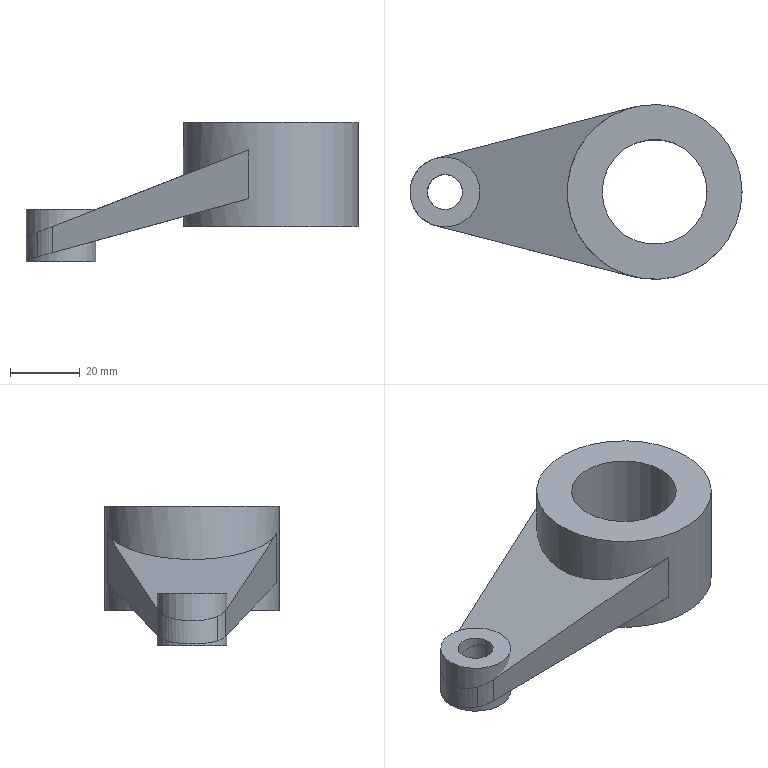Part | NX | features DATUM_CSYS 7, EXTRUDE 6, SKETCH 6, REPLACE_FACE 5, DATUM_PLANE 2 | 2 solids | 15 faces | box 95 x 50 x 40 mm | volume 53901 mm3 | plane 8 | cylinder 7 | commonest cylinder face diameters 20 x3 10 x2 30 x1 50 x1
STEP:
#1=CARTESIAN_POINT('',(5.,0.,13.029));
#2=VERTEX_POINT('',#1);
#3=CARTESIAN_POINT('',(0.,0.,11.079));
#4=DIRECTION('',(0.3634,0.,-0.9316));
#5=DIRECTION('',(0.9316,0.,0.3634));
#6=AXIS2_PLACEMENT_3D('',#3,#4,#5);
#7=ELLIPSE('',#6,5.367,5.);
#8=EDGE_CURVE('',#2,#2,#7,.F.);
#9=ORIENTED_EDGE('',*,*,#8,.F.);
#10=EDGE_LOOP('',(#9));
#11=FACE_BOUND('',#10,.T.);
#12=CARTESIAN_POINT('',(53.75,-24.206,32.048));
#13=VERTEX_POINT('',#12);
#14=CARTESIAN_POINT('',(53.75,24.206,32.048));
#15=VERTEX_POINT('',#14);
#16=CARTESIAN_POINT('',(60.,0.,34.486));
#17=DIRECTION('',(0.3634,0.,-0.9316));
#18=DIRECTION('',(-0.9316,0.,-0.3634));
#19=AXIS2_PLACEMENT_3D('',#16,#17,#18);
#20=ELLIPSE('',#19,26.835,25.);
#21=EDGE_CURVE('',#13,#15,#20,.T.);
#22=ORIENTED_EDGE('',*,*,#21,.T.);
#23=CARTESIAN_POINT('',(-2.5,9.682,10.103));
#24=VERTEX_POINT('',#23);
#25=CARTESIAN_POINT('',(-24.938,3.889,1.35));
#26=DIRECTION('',(0.9058,0.2339,0.3534));
#27=VECTOR('',#26,1000.);
#28=LINE('',#25,#27);
#29=EDGE_CURVE('',#24,#15,#28,.T.);
#30=ORIENTED_EDGE('',*,*,#29,.F.);
#31=CARTESIAN_POINT('',(-6.747,-7.381,8.447));
#32=VERTEX_POINT('',#31);
#33=CARTESIAN_POINT('',(0.,0.,11.079));
#34=DIRECTION('',(0.3634,0.,-0.9316));
#35=DIRECTION('',(-0.9316,0.,-0.3634));
#36=AXIS2_PLACEMENT_3D('',#33,#34,#35);
#37=ELLIPSE('',#36,10.734,10.);
#38=EDGE_CURVE('',#24,#32,#37,.F.);
#39=ORIENTED_EDGE('',*,*,#38,.T.);
#40=CARTESIAN_POINT('',(-2.5,-9.682,10.103));
#41=VERTEX_POINT('',#40);
#42=CARTESIAN_POINT('',(0.,0.,11.079));
#43=DIRECTION('',(0.3634,0.,-0.9316));
#44=DIRECTION('',(-0.9316,0.,-0.3634));
#45=AXIS2_PLACEMENT_3D('',#42,#43,#44);
#46=ELLIPSE('',#45,10.734,10.);
#47=EDGE_CURVE('',#32,#41,#46,.F.);
#48=ORIENTED_EDGE('',*,*,#47,.T.);
#49=CARTESIAN_POINT('',(-14.921,-6.475,5.258));
#50=DIRECTION('',(0.9058,-0.2339,0.3534));
#51=VECTOR('',#50,1000.);
#52=LINE('',#49,#51);
#53=EDGE_CURVE('',#41,#13,#52,.T.);
#54=ORIENTED_EDGE('',*,*,#53,.T.);
#55=EDGE_LOOP('',(#22,#30,#39,#48,#54));
#56=FACE_BOUND('',#55,.T.);
#57=CARTESIAN_POINT('',(-6.747,30.,8.447));
#58=DIRECTION('',(0.3634,0.,-0.9316));
#59=DIRECTION('',(-0.9316,0.,-0.3634));
#60=AXIS2_PLACEMENT_3D('',#57,#58,#59);
#61=PLANE('',#60);
#62=ADVANCED_FACE('',(#11,#56),#61,.F.);
#63=CARTESIAN_POINT('',(5.,0.,4.697));
#64=VERTEX_POINT('',#63);
#65=CARTESIAN_POINT('',(0.,0.,3.321));
#66=DIRECTION('',(-0.2654,0.,0.9641));
#67=DIRECTION('',(0.9641,0.,0.2654));
#68=AXIS2_PLACEMENT_3D('',#65,#66,#67);
#69=ELLIPSE('',#68,5.186,5.);
#70=EDGE_CURVE('',#64,#64,#69,.F.);
#71=ORIENTED_EDGE('',*,*,#70,.F.);
#72=EDGE_LOOP('',(#71));
#73=FACE_BOUND('',#72,.T.);
#74=CARTESIAN_POINT('',(53.75,24.206,18.117));
#75=VERTEX_POINT('',#74);
#76=CARTESIAN_POINT('',(-2.5,9.682,2.633));
#77=VERTEX_POINT('',#76);
#78=CARTESIAN_POINT('',(-17.591,5.786,-1.522));
#79=DIRECTION('',(-0.9356,-0.2416,-0.2575));
#80=VECTOR('',#79,1000.);
#81=LINE('',#78,#80);
#82=EDGE_CURVE('',#75,#77,#81,.T.);
#83=ORIENTED_EDGE('',*,*,#82,.F.);
#84=CARTESIAN_POINT('',(53.75,-24.206,18.117));
#85=VERTEX_POINT('',#84);
#86=CARTESIAN_POINT('',(60.,0.,19.837));
#87=DIRECTION('',(-0.2654,0.,0.9641));
#88=DIRECTION('',(-0.9641,0.,-0.2654));
#89=AXIS2_PLACEMENT_3D('',#86,#87,#88);
#90=ELLIPSE('',#89,25.93,25.);
#91=EDGE_CURVE('',#75,#85,#90,.T.);
#92=ORIENTED_EDGE('',*,*,#91,.T.);
#93=CARTESIAN_POINT('',(-2.5,-9.682,2.633));
#94=VERTEX_POINT('',#93);
#95=CARTESIAN_POINT('',(57.593,-25.198,19.175));
#96=DIRECTION('',(-0.9356,0.2416,-0.2575));
#97=VECTOR('',#96,1000.);
#98=LINE('',#95,#97);
#99=EDGE_CURVE('',#85,#94,#98,.T.);
#100=ORIENTED_EDGE('',*,*,#99,.T.);
#101=CARTESIAN_POINT('',(-6.747,-7.381,1.464));
#102=VERTEX_POINT('',#101);
#103=CARTESIAN_POINT('',(0.,0.,3.321));
#104=DIRECTION('',(-0.2654,0.,0.9641));
#105=DIRECTION('',(-0.9641,0.,-0.2654));
#106=AXIS2_PLACEMENT_3D('',#103,#104,#105);
#107=ELLIPSE('',#106,10.372,10.);
#108=EDGE_CURVE('',#94,#102,#107,.F.);
#109=ORIENTED_EDGE('',*,*,#108,.T.);
#110=CARTESIAN_POINT('',(0.,0.,3.321));
#111=DIRECTION('',(-0.2654,0.,0.9641));
#112=DIRECTION('',(-0.9641,0.,-0.2654));
#113=AXIS2_PLACEMENT_3D('',#110,#111,#112);
#114=ELLIPSE('',#113,10.372,10.);
#115=EDGE_CURVE('',#77,#102,#114,.T.);
#116=ORIENTED_EDGE('',*,*,#115,.F.);
#117=EDGE_LOOP('',(#83,#92,#100,#109,#116));
#118=FACE_BOUND('',#117,.T.);
#119=CARTESIAN_POINT('',(70.841,30.,22.822));
#120=DIRECTION('',(-0.2654,0.,0.9641));
#121=DIRECTION('',(0.9641,0.,0.2654));
#122=AXIS2_PLACEMENT_3D('',#119,#120,#121);
#123=PLANE('',#122);
#124=ADVANCED_FACE('',(#73,#118),#123,.F.);
#125=CARTESIAN_POINT('',(53.75,24.206,30.769));
#126=DIRECTION('',(0.,0.,-1.));
#127=VECTOR('',#126,1000.);
#128=LINE('',#125,#127);
#129=EDGE_CURVE('',#15,#75,#128,.T.);
#130=ORIENTED_EDGE('',*,*,#129,.F.);
#131=ORIENTED_EDGE('',*,*,#21,.F.);
#132=CARTESIAN_POINT('',(53.75,-24.206,30.769));
#133=DIRECTION('',(0.,0.,-1.));
#134=VECTOR('',#133,1000.);
#135=LINE('',#132,#134);
#136=EDGE_CURVE('',#13,#85,#135,.T.);
#137=ORIENTED_EDGE('',*,*,#136,.T.);
#138=ORIENTED_EDGE('',*,*,#91,.F.);
#139=EDGE_LOOP('',(#130,#131,#137,#138));
#140=FACE_BOUND('',#139,.T.);
#141=CARTESIAN_POINT('',(85.,0.,10.));
#142=VERTEX_POINT('',#141);
#143=CARTESIAN_POINT('',(60.,0.,10.));
#144=DIRECTION('',(0.,0.,1.));
#145=DIRECTION('',(1.,0.,0.));
#146=AXIS2_PLACEMENT_3D('',#143,#144,#145);
#147=CIRCLE('',#146,25.);
#148=EDGE_CURVE('',#142,#142,#147,.T.);
#149=ORIENTED_EDGE('',*,*,#148,.T.);
#150=EDGE_LOOP('',(#149));
#151=FACE_BOUND('',#150,.T.);
#152=CARTESIAN_POINT('',(85.,0.,40.));
#153=VERTEX_POINT('',#152);
#154=CARTESIAN_POINT('',(60.,0.,40.));
#155=DIRECTION('',(0.,0.,1.));
#156=DIRECTION('',(1.,0.,0.));
#157=AXIS2_PLACEMENT_3D('',#154,#155,#156);
#158=CIRCLE('',#157,25.);
#159=EDGE_CURVE('',#153,#153,#158,.T.);
#160=ORIENTED_EDGE('',*,*,#159,.F.);
#161=EDGE_LOOP('',(#160));
#162=FACE_BOUND('',#161,.T.);
#163=CARTESIAN_POINT('',(60.,0.,40.));
#164=DIRECTION('',(0.,0.,-1.));
#165=DIRECTION('',(-1.,0.,0.));
#166=AXIS2_PLACEMENT_3D('',#163,#164,#165);
#167=CYLINDRICAL_SURFACE('',#166,25.);
#168=ADVANCED_FACE('',(#140,#151,#162),#167,.T.);
#169=CARTESIAN_POINT('',(75.,0.,40.));
#170=VERTEX_POINT('',#169);
#171=CARTESIAN_POINT('',(60.,0.,40.));
#172=DIRECTION('',(0.,0.,1.));
#173=DIRECTION('',(1.,0.,0.));
#174=AXIS2_PLACEMENT_3D('',#171,#172,#173);
#175=CIRCLE('',#174,15.);
#176=EDGE_CURVE('',#170,#170,#175,.T.);
#177=ORIENTED_EDGE('',*,*,#176,.T.);
#178=EDGE_LOOP('',(#177));
#179=FACE_BOUND('',#178,.T.);
#180=CARTESIAN_POINT('',(75.,0.,10.));
#181=VERTEX_POINT('',#180);
#182=CARTESIAN_POINT('',(60.,0.,10.));
#183=DIRECTION('',(0.,0.,1.));
#184=DIRECTION('',(1.,0.,0.));
#185=AXIS2_PLACEMENT_3D('',#182,#183,#184);
#186=CIRCLE('',#185,15.);
#187=EDGE_CURVE('',#181,#181,#186,.T.);
#188=ORIENTED_EDGE('',*,*,#187,.F.);
#189=EDGE_LOOP('',(#188));
#190=FACE_BOUND('',#189,.T.);
#191=CARTESIAN_POINT('',(60.,0.,40.));
#192=DIRECTION('',(0.,0.,-1.));
#193=DIRECTION('',(-1.,0.,0.));
#194=AXIS2_PLACEMENT_3D('',#191,#192,#193);
#195=CYLINDRICAL_SURFACE('',#194,15.);
#196=ADVANCED_FACE('',(#179,#190),#195,.F.);
#197=ORIENTED_EDGE('',*,*,#159,.T.);
#198=EDGE_LOOP('',(#197));
#199=FACE_BOUND('',#198,.T.);
#200=ORIENTED_EDGE('',*,*,#176,.F.);
#201=EDGE_LOOP('',(#200));
#202=FACE_BOUND('',#201,.T.);
#203=CARTESIAN_POINT('',(60.,0.,40.));
#204=DIRECTION('',(0.,0.,1.));
#205=DIRECTION('',(1.,0.,0.));
#206=AXIS2_PLACEMENT_3D('',#203,#204,#205);
#207=PLANE('',#206);
#208=ADVANCED_FACE('',(#199,#202),#207,.T.);
#209=ORIENTED_EDGE('',*,*,#148,.F.);
#210=EDGE_LOOP('',(#209));
#211=FACE_BOUND('',#210,.T.);
#212=ORIENTED_EDGE('',*,*,#187,.T.);
#213=EDGE_LOOP('',(#212));
#214=FACE_BOUND('',#213,.T.);
#215=CARTESIAN_POINT('',(60.,0.,10.));
#216=DIRECTION('',(0.,0.,1.));
#217=DIRECTION('',(1.,0.,0.));
#218=AXIS2_PLACEMENT_3D('',#215,#216,#217);
#219=PLANE('',#218);
#220=ADVANCED_FACE('',(#211,#214),#219,.F.);
#221=CARTESIAN_POINT('',(-6.747,-7.381,4.955));
#222=DIRECTION('',(0.,0.,-1.));
#223=VECTOR('',#222,1000.);
#224=LINE('',#221,#223);
#225=EDGE_CURVE('',#102,#32,#224,.F.);
#226=ORIENTED_EDGE('',*,*,#225,.T.);
#227=ORIENTED_EDGE('',*,*,#38,.F.);
#228=CARTESIAN_POINT('',(-2.5,9.682,4.955));
#229=DIRECTION('',(0.,0.,-1.));
#230=VECTOR('',#229,1000.);
#231=LINE('',#228,#230);
#232=EDGE_CURVE('',#77,#24,#231,.F.);
#233=ORIENTED_EDGE('',*,*,#232,.F.);
#234=ORIENTED_EDGE('',*,*,#115,.T.);
#235=EDGE_LOOP('',(#226,#227,#233,#234));
#236=FACE_BOUND('',#235,.T.);
#237=CARTESIAN_POINT('',(0.,0.,15.));
#238=DIRECTION('',(0.,0.,-1.));
#239=DIRECTION('',(-1.,0.,0.));
#240=AXIS2_PLACEMENT_3D('',#237,#238,#239);
#241=CYLINDRICAL_SURFACE('',#240,10.);
#242=ADVANCED_FACE('',(#236),#241,.T.);
#243=ORIENTED_EDGE('',*,*,#29,.T.);
#244=ORIENTED_EDGE('',*,*,#129,.T.);
#245=ORIENTED_EDGE('',*,*,#82,.T.);
#246=ORIENTED_EDGE('',*,*,#232,.T.);
#247=EDGE_LOOP('',(#243,#244,#245,#246));
#248=FACE_BOUND('',#247,.T.);
#249=CARTESIAN_POINT('',(-2.5,9.682,-60.));
#250=DIRECTION('',(0.25,-0.9682,0.));
#251=DIRECTION('',(0.9682,0.25,0.));
#252=AXIS2_PLACEMENT_3D('',#249,#250,#251);
#253=PLANE('',#252);
#254=ADVANCED_FACE('',(#248),#253,.F.);
#255=CARTESIAN_POINT('',(-2.5,-9.682,-60.));
#256=DIRECTION('',(0.,0.,1.));
#257=VECTOR('',#256,1000.);
#258=LINE('',#255,#257);
#259=EDGE_CURVE('',#41,#94,#258,.F.);
#260=ORIENTED_EDGE('',*,*,#259,.F.);
#261=ORIENTED_EDGE('',*,*,#47,.F.);
#262=ORIENTED_EDGE('',*,*,#225,.F.);
#263=ORIENTED_EDGE('',*,*,#108,.F.);
#264=EDGE_LOOP('',(#260,#261,#262,#263));
#265=FACE_BOUND('',#264,.T.);
#266=CARTESIAN_POINT('',(0.,0.,15.));
#267=DIRECTION('',(0.,0.,-1.));
#268=DIRECTION('',(-1.,0.,0.));
#269=AXIS2_PLACEMENT_3D('',#266,#267,#268);
#270=CYLINDRICAL_SURFACE('',#269,10.);
#271=ADVANCED_FACE('',(#265),#270,.T.);
#272=ORIENTED_EDGE('',*,*,#259,.T.);
#273=ORIENTED_EDGE('',*,*,#99,.F.);
#274=ORIENTED_EDGE('',*,*,#136,.F.);
#275=ORIENTED_EDGE('',*,*,#53,.F.);
#276=EDGE_LOOP('',(#272,#273,#274,#275));
#277=FACE_BOUND('',#276,.T.);
#278=CARTESIAN_POINT('',(98.431,-35.743,-60.));
#279=DIRECTION('',(0.25,0.9682,0.));
#280=DIRECTION('',(-0.9682,0.25,0.));
#281=AXIS2_PLACEMENT_3D('',#278,#279,#280);
#282=PLANE('',#281);
#283=ADVANCED_FACE('',(#277),#282,.F.);
#284=ORIENTED_EDGE('',*,*,#70,.T.);
#285=EDGE_LOOP('',(#284));
#286=FACE_BOUND('',#285,.T.);
#287=ORIENTED_EDGE('',*,*,#8,.T.);
#288=EDGE_LOOP('',(#287));
#289=FACE_BOUND('',#288,.T.);
#290=CARTESIAN_POINT('',(0.,0.,-85.));
#291=DIRECTION('',(0.,0.,1.));
#292=DIRECTION('',(1.,0.,0.));
#293=AXIS2_PLACEMENT_3D('',#290,#291,#292);
#294=CYLINDRICAL_SURFACE('',#293,5.);
#295=ADVANCED_FACE('',(#286,#289),#294,.F.);
#296=CLOSED_SHELL('',(#62,#124,#168,#196,#208,#220,#242,#254,#271,#283,#295));
#297=MANIFOLD_SOLID_BREP('',#296);
#298=CARTESIAN_POINT('',(10.,0.,15.));
#299=VERTEX_POINT('',#298);
#300=CARTESIAN_POINT('',(0.,0.,15.));
#301=DIRECTION('',(0.,0.,1.));
#302=DIRECTION('',(1.,0.,0.));
#303=AXIS2_PLACEMENT_3D('',#300,#301,#302);
#304=CIRCLE('',#303,10.);
#305=EDGE_CURVE('',#299,#299,#304,.T.);
#306=ORIENTED_EDGE('',*,*,#305,.F.);
#307=EDGE_LOOP('',(#306));
#308=FACE_BOUND('',#307,.T.);
#309=CARTESIAN_POINT('',(10.,0.,0.));
#310=VERTEX_POINT('',#309);
#311=CARTESIAN_POINT('',(0.,0.,0.));
#312=DIRECTION('',(0.,0.,1.));
#313=DIRECTION('',(1.,0.,0.));
#314=AXIS2_PLACEMENT_3D('',#311,#312,#313);
#315=CIRCLE('',#314,10.);
#316=EDGE_CURVE('',#310,#310,#315,.T.);
#317=ORIENTED_EDGE('',*,*,#316,.T.);
#318=EDGE_LOOP('',(#317));
#319=FACE_BOUND('',#318,.T.);
#320=CARTESIAN_POINT('',(0.,0.,15.));
#321=DIRECTION('',(0.,0.,-1.));
#322=DIRECTION('',(-1.,0.,0.));
#323=AXIS2_PLACEMENT_3D('',#320,#321,#322);
#324=CYLINDRICAL_SURFACE('',#323,10.);
#325=ADVANCED_FACE('',(#308,#319),#324,.T.);
#326=CARTESIAN_POINT('',(5.,0.,15.));
#327=VERTEX_POINT('',#326);
#328=CARTESIAN_POINT('',(0.,0.,15.));
#329=DIRECTION('',(0.,0.,1.));
#330=DIRECTION('',(1.,0.,0.));
#331=AXIS2_PLACEMENT_3D('',#328,#329,#330);
#332=CIRCLE('',#331,5.);
#333=EDGE_CURVE('',#327,#327,#332,.T.);
#334=ORIENTED_EDGE('',*,*,#333,.T.);
#335=EDGE_LOOP('',(#334));
#336=FACE_BOUND('',#335,.T.);
#337=CARTESIAN_POINT('',(5.,0.,0.));
#338=VERTEX_POINT('',#337);
#339=CARTESIAN_POINT('',(0.,0.,0.));
#340=DIRECTION('',(0.,0.,1.));
#341=DIRECTION('',(1.,0.,0.));
#342=AXIS2_PLACEMENT_3D('',#339,#340,#341);
#343=CIRCLE('',#342,5.);
#344=EDGE_CURVE('',#338,#338,#343,.T.);
#345=ORIENTED_EDGE('',*,*,#344,.F.);
#346=EDGE_LOOP('',(#345));
#347=FACE_BOUND('',#346,.T.);
#348=CARTESIAN_POINT('',(0.,0.,15.));
#349=DIRECTION('',(0.,0.,-1.));
#350=DIRECTION('',(-1.,0.,0.));
#351=AXIS2_PLACEMENT_3D('',#348,#349,#350);
#352=CYLINDRICAL_SURFACE('',#351,5.);
#353=ADVANCED_FACE('',(#336,#347),#352,.F.);
#354=ORIENTED_EDGE('',*,*,#305,.T.);
#355=EDGE_LOOP('',(#354));
#356=FACE_BOUND('',#355,.T.);
#357=ORIENTED_EDGE('',*,*,#333,.F.);
#358=EDGE_LOOP('',(#357));
#359=FACE_BOUND('',#358,.T.);
#360=CARTESIAN_POINT('',(0.,0.,15.));
#361=DIRECTION('',(0.,0.,1.));
#362=DIRECTION('',(1.,0.,0.));
#363=AXIS2_PLACEMENT_3D('',#360,#361,#362);
#364=PLANE('',#363);
#365=ADVANCED_FACE('',(#356,#359),#364,.T.);
#366=ORIENTED_EDGE('',*,*,#316,.F.);
#367=EDGE_LOOP('',(#366));
#368=FACE_BOUND('',#367,.T.);
#369=ORIENTED_EDGE('',*,*,#344,.T.);
#370=EDGE_LOOP('',(#369));
#371=FACE_BOUND('',#370,.T.);
#372=CARTESIAN_POINT('',(0.,0.,0.));
#373=DIRECTION('',(0.,0.,1.));
#374=DIRECTION('',(1.,0.,0.));
#375=AXIS2_PLACEMENT_3D('',#372,#373,#374);
#376=PLANE('',#375);
#377=ADVANCED_FACE('',(#368,#371),#376,.F.);
#378=CLOSED_SHELL('',(#325,#353,#365,#377));
#379=MANIFOLD_SOLID_BREP('',#378);
#380=(LENGTH_UNIT()NAMED_UNIT(*)SI_UNIT(.MILLI.,.METRE.));
#381=UNCERTAINTY_MEASURE_WITH_UNIT(LENGTH_MEASURE(0.00001),#380,'','');
#382=(NAMED_UNIT(*)PLANE_ANGLE_UNIT()SI_UNIT($,.RADIAN.));
#383=(NAMED_UNIT(*)SI_UNIT($,.STERADIAN.)SOLID_ANGLE_UNIT());
#384=(GEOMETRIC_REPRESENTATION_CONTEXT(3)GLOBAL_UNCERTAINTY_ASSIGNED_CONTEXT((#381))GLOBAL_UNIT_ASSIGNED_CONTEXT((#380,#382,#383))REPRESENTATION_CONTEXT('',''));
#385=ADVANCED_BREP_SHAPE_REPRESENTATION('',(#297,#379),#384);